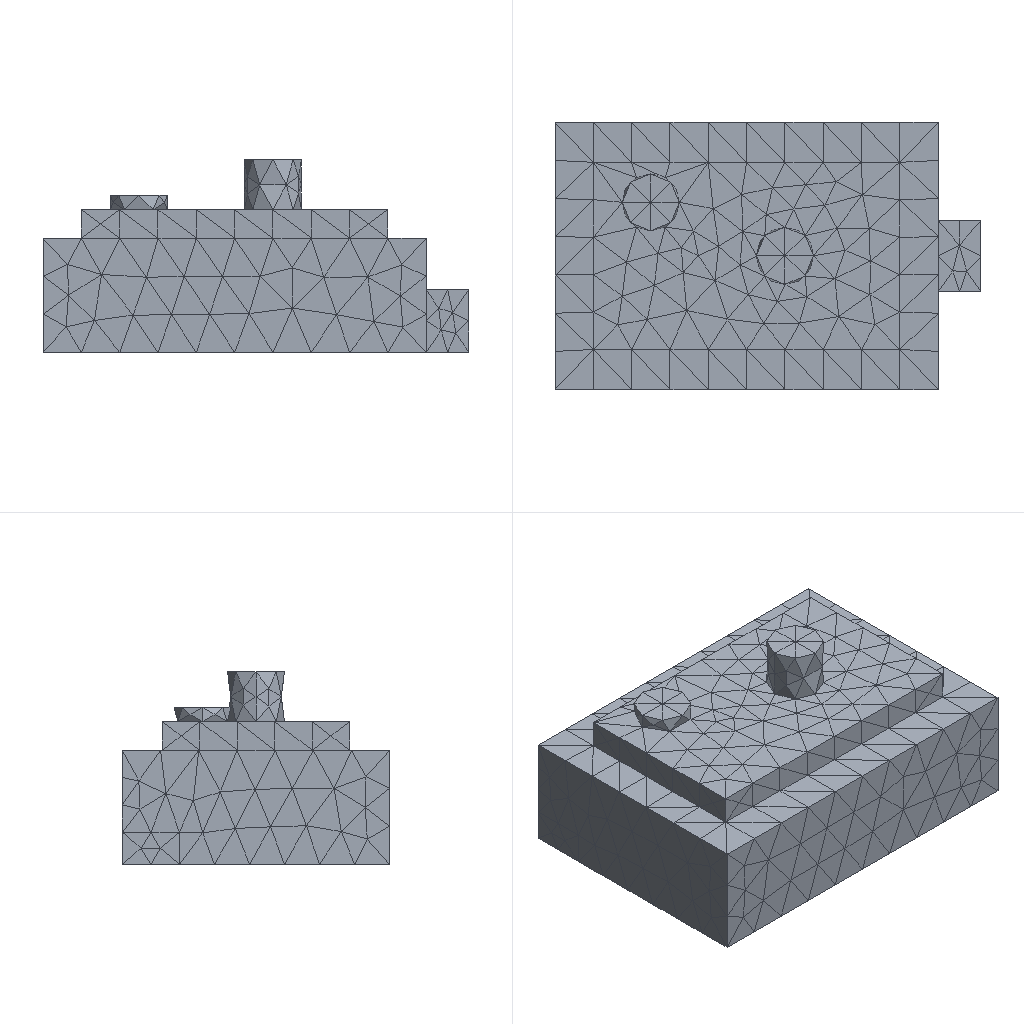Simulation study | ansys mapdl
Set-up summary:
category,name,step,type,value,unit,region
solver,ansys_mapdl
units,mm-N-s-tonne (MPa),,inferred,E=210000 density=
analysis,model,,static
mesh,nodes,,,4457
mesh,elements,,,2653
element_type,SOLID187,,,2653
material,mat 1,,E,210000
material,mat 1,,nu,0.3
load,,model,body load temp,,,all
load,,model,force,"1000 [dir=(0, 0, -1) n=126]",,node list
bc,,model,fixed,"[dofs=UX,UY,UZ n=4681]",,node list
Ansys APDL input file, long lists of numbers shortened:
/COM,ANSYS RELEASE 2026 R1           BUILD 26.1      UP20260202       09:10:32
/PREP7
/NOPR
/TITLE,2
ANTYPE, 0
*IF,_CDRDOFF,EQ,1,THEN     !if solid model was read in
_CDRDOFF=             !reset flag, numoffs already performed
*ELSE              !offset database for the following FE model
NUMOFF,NODE,     4457
NUMOFF,ELEM,     2653
NUMOFF,MAT ,        1
NUMOFF,TYPE,        1
*ENDIF
*SET,_RETURN ,  0.
*SET,_STATUS ,  0.
*SET,_UIQR   ,  126.
*SET,__FLOATPARAMETER__,  4457.
DOF,DELETE
ETBLOCK,        1,        1
(2i9,19a9)
        1      187        0        0        0        0        0        0        0        0        0        0        0        0        0        0        0        0        0        0        0
       -1
NBLOCK,6,SOLID,      4457,      4457
(3i9,6e21.13e3)
        1        0        0-3.7750000000000E+001 3.7500000000000E+001 9.0000000000000E+000
! (4456 more lines like these left out)
N,UNBL,LOC,       -1,
EBLOCK,19,SOLID,      2653,      2653
(19i10)
         1         1         1         1         0         0         0         0        10         0         1      1502        46      1735      1142      1176      1986      1987      1988
! (5305 more lines like these left out)
        -1
MPTEMP,UNBL, 1, 1,  0.    ,
MPDATA,UNBL, 1,EX  ,       1, 1,  210000.000    ,
MPTEMP,UNBL, 1, 1,  0.    ,
MPDATA,UNBL, 1,NUXY,       1, 1, 0.3    ,
MPTEMP,UNBL, 1, 1,  0.    ,
MPDATA,UNBL, 1,PRXY,       1, 1, 0.3    ,
EXTOPT,ATTR,      0,      0,      0
EXTOPT,ESIZE,  0,  0.
EXTOPT,ACLEAR,      0
TREF,  0.
IRLF,  0
BFUNIF,TEMP,_TINY
ACEL,  0.    ,  0.    ,  0.
OMEGA,  0.    ,  0.    ,  0.
DOMEGA,  0.    ,  0.    ,  0.
CGLOC,  0.    ,  0.    ,  0.
CGOMEGA,  0.    ,  0.    ,  0.
DCGOMG,  0.    ,  0.    ,  0.
KUSE,     0
TIME,  0.
ALPHAD,  0.
BETAD,  0.
DMPRAT,  0.
DMPSTR,  0.
CRPLIM, 0.1    ,   0
CRPLIM,  0.    ,   1
NCNV,     0, 1.000000000E+12,     0,  0.    ,  0.
NEQIT,     0
ERESX,DEFA
DBLOCK,      4681
(i9,a6,2(pg16.9))
        1  UX    0.00000000      0.00000000
! (4680 more lines like these left out)
       -1
FBLOCK,       126
(i9,a6,2(pg16.9))
      870  FZ   -7.93650794      0.00000000
! (125 more lines like these left out)
       -1
/GO
FINISH
Results summary:
result,analysis_type_db,,,static,unstated
result,n_sets,,,1,unstated
result,load_steps[0].set,load_step=1,,1,unstated
result,load_steps[0].substep,load_step=1,,1,unstated
result,load_steps[0].time,load_step=1,,1,unstated
result,load_steps[0].freq,load_step=1,,1,unstated
result,load_steps[0].max_usum,load_step=1,,0.000476,unstated
result,load_steps[0].max_seqv,load_step=1,,5.871,unstated
result,load_steps[0].reaction_sum.FX,load_step=1,,1.25695e-11,unstated
result,load_steps[0].reaction_sum.FY,load_step=1,,-3.38929e-12,unstated
result,load_steps[0].reaction_sum.FZ,load_step=1,,1000,unstated
result,load_steps[0].reaction_sum.MX,load_step=1,,0,unstated
result,load_steps[0].reaction_sum.MY,load_step=1,,0,unstated
result,load_steps[0].reaction_sum.MZ,load_step=1,,0,unstated
result,convergence,,,results present for all listed sets,unstated